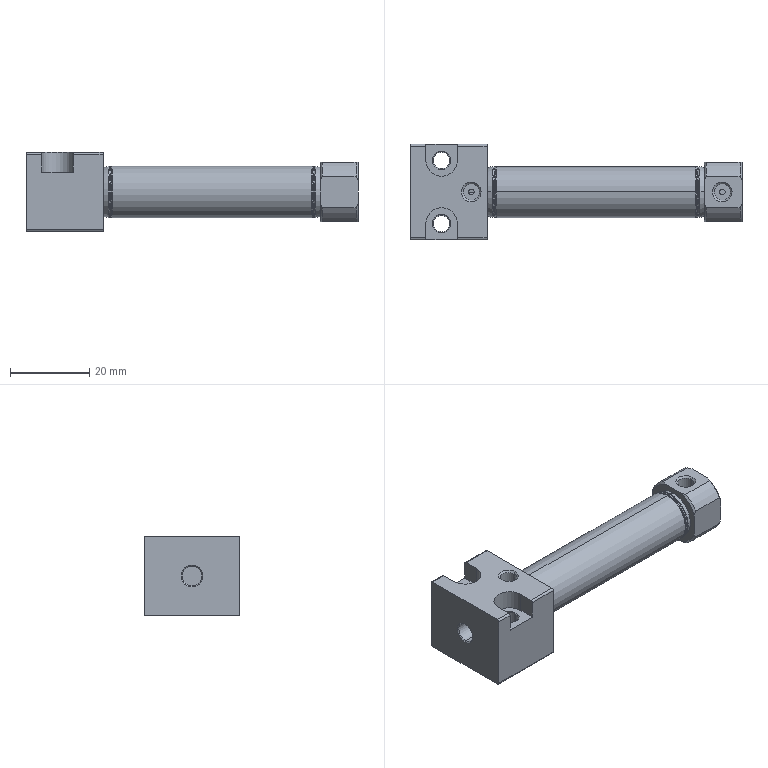Part | STEP file | PBR12X30SU-01-CC | 1 solid | 114 faces | box 84 x 24.2 x 20 mm | volume 10911 mm3 | cylinder 36 | cone 36 | plane 26 | spline 16 | commonest cylinder face diameters 4.134 x8 1 x6 1.5 x4 4.3 x4 17 x4 5 x2